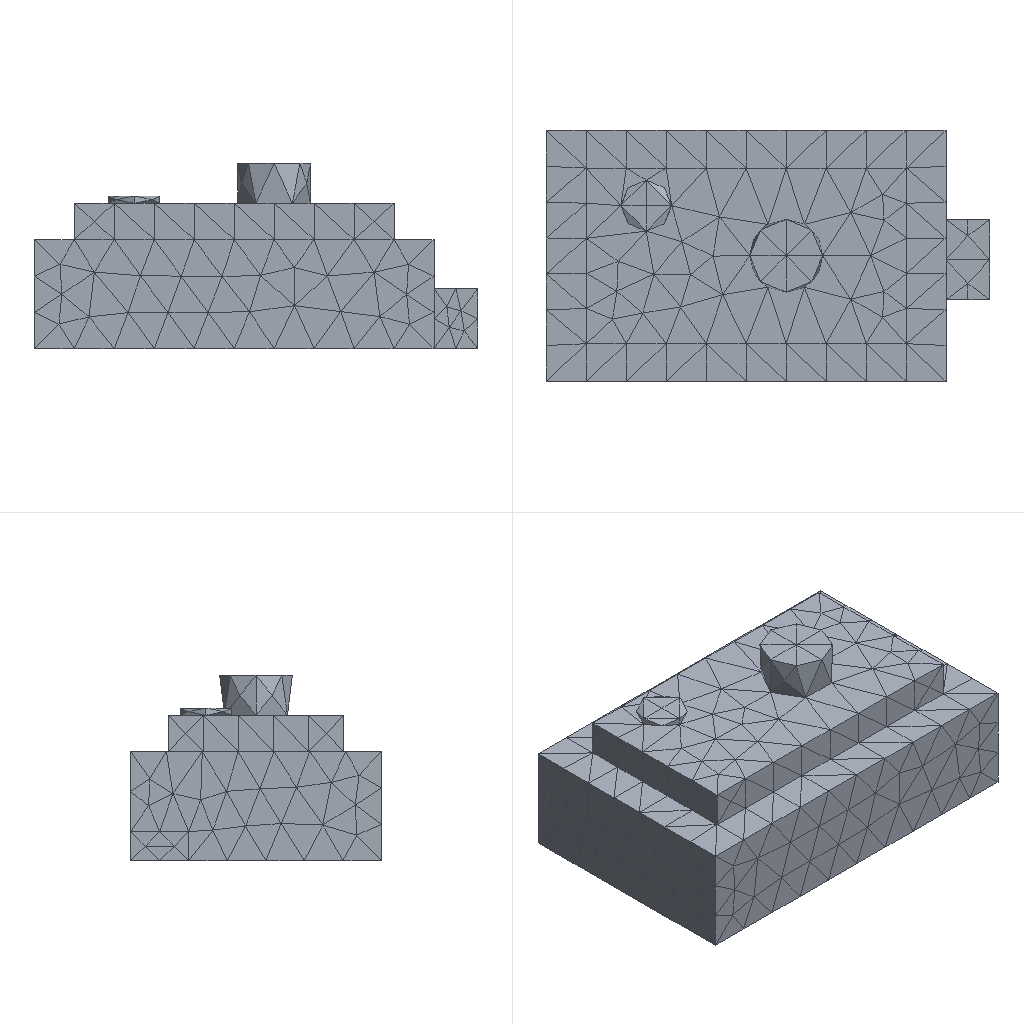Simulation study | ansys mapdl
Set-up summary:
category,name,step,type,value,unit,region
solver,ansys_mapdl
units,mm-N-s-tonne (MPa),,inferred,E=210000 density=
analysis,model,,static
mesh,nodes,,,3482
mesh,elements,,,2017
element_type,SOLID187,,,2017
material,mat 1,,E,210000
material,mat 1,,nu,0.3
load,,model,body load temp,,,all
load,,model,force,"1000 [dir=(0, 0, -1) n=78]",,node list
bc,,model,fixed,"[dofs=UX,UY,UZ n=3914]",,node list
Ansys APDL input file, long lists of numbers shortened:
/COM,ANSYS RELEASE 2026 R1           BUILD 26.1      UP20260202       09:08:28
/PREP7
/NOPR
/TITLE,2
ANTYPE, 0
*IF,_CDRDOFF,EQ,1,THEN     !if solid model was read in
_CDRDOFF=             !reset flag, numoffs already performed
*ELSE              !offset database for the following FE model
NUMOFF,NODE,     3482
NUMOFF,ELEM,     2017
NUMOFF,MAT ,        1
NUMOFF,TYPE,        1
*ENDIF
*SET,_RETURN ,  0.
*SET,_STATUS ,  0.
*SET,_UIQR   ,  78.
*SET,__FLOATPARAMETER__,  3482.
DOF,DELETE
ETBLOCK,        1,        1
(2i9,19a9)
        1      187        0        0        0        0        0        0        0        0        0        0        0        0        0        0        0        0        0        0        0
       -1
NBLOCK,6,SOLID,      3482,      3482
(3i9,6e21.13e3)
        1        0        0-3.8975000000000E+001 3.4500000000000E+001 8.0000000000000E+000
! (3481 more lines like these left out)
N,UNBL,LOC,       -1,
EBLOCK,19,SOLID,      2017,      2017
(19i10)
         1         1         1         1         0         0         0         0        10         0         1      1491      1492      1493      1494      1664      1665      1666      1667
! (4033 more lines like these left out)
        -1
MPTEMP,UNBL, 1, 1,  0.    ,
MPDATA,UNBL, 1,EX  ,       1, 1,  210000.000    ,
MPTEMP,UNBL, 1, 1,  0.    ,
MPDATA,UNBL, 1,NUXY,       1, 1, 0.3    ,
MPTEMP,UNBL, 1, 1,  0.    ,
MPDATA,UNBL, 1,PRXY,       1, 1, 0.3    ,
EXTOPT,ATTR,      0,      0,      0
EXTOPT,ESIZE,  0,  0.
EXTOPT,ACLEAR,      0
TREF,  0.
IRLF,  0
BFUNIF,TEMP,_TINY
ACEL,  0.    ,  0.    ,  0.
OMEGA,  0.    ,  0.    ,  0.
DOMEGA,  0.    ,  0.    ,  0.
CGLOC,  0.    ,  0.    ,  0.
CGOMEGA,  0.    ,  0.    ,  0.
DCGOMG,  0.    ,  0.    ,  0.
KUSE,     0
TIME,  0.
ALPHAD,  0.
BETAD,  0.
DMPRAT,  0.
DMPSTR,  0.
CRPLIM, 0.1    ,   0
CRPLIM,  0.    ,   1
NCNV,     0, 1.000000000E+12,     0,  0.    ,  0.
NEQIT,     0
ERESX,DEFA
DBLOCK,      3914
(i9,a6,2(pg16.9))
        1  UX    0.00000000      0.00000000
! (3913 more lines like these left out)
       -1
FBLOCK,        78
(i9,a6,2(pg16.9))
      713  FZ   -12.8205128      0.00000000
! (77 more lines like these left out)
       -1
/GO
FINISH
Results summary:
result,analysis_type_db,,,static,unstated
result,n_sets,,,1,unstated
result,load_steps[0].set,load_step=1,,1,unstated
result,load_steps[0].substep,load_step=1,,1,unstated
result,load_steps[0].time,load_step=1,,1,unstated
result,load_steps[0].freq,load_step=1,,1,unstated
result,load_steps[0].max_usum,load_step=1,,0.0003066,unstated
result,load_steps[0].max_seqv,load_step=1,,3.628,unstated
result,load_steps[0].reaction_sum.FX,load_step=1,,4.94182e-12,unstated
result,load_steps[0].reaction_sum.FY,load_step=1,,-4.28546e-13,unstated
result,load_steps[0].reaction_sum.FZ,load_step=1,,1000,unstated
result,load_steps[0].reaction_sum.MX,load_step=1,,0,unstated
result,load_steps[0].reaction_sum.MY,load_step=1,,0,unstated
result,load_steps[0].reaction_sum.MZ,load_step=1,,0,unstated
result,convergence,,,results present for all listed sets,unstated